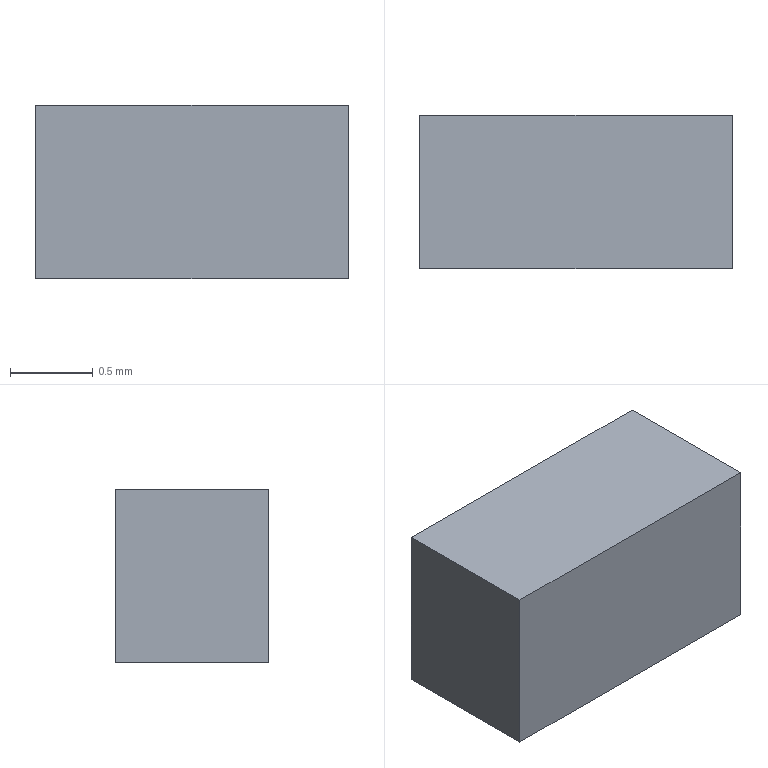Part | Creo | 1 solid | 6 faces | box 1.889 x 0.9288 x 1.053 mm | volume 1.848 mm3 | plane 6
STEP:
#1=CARTESIAN_POINT('',(0.,0.,0.));
#2=DIRECTION('',(0.,0.,1.));
#3=DIRECTION('',(1.,0.,0.));
#4=AXIS2_PLACEMENT_3D('',#1,#2,#3);
#5=CARTESIAN_POINT('',(-0.9404,-0.4484,0.));
#6=VERTEX_POINT('',#5);
#7=CARTESIAN_POINT('',(0.9491,-0.4484,0.));
#8=VERTEX_POINT('',#7);
#9=CARTESIAN_POINT('',(-0.9404,-0.4484,0.));
#10=DIRECTION('',(1.,0.,0.));
#11=VECTOR('',#10,1.889);
#12=LINE('',#9,#11);
#13=EDGE_CURVE('',#6,#8,#12,.T.);
#14=ORIENTED_EDGE('',*,*,#13,.T.);
#15=CARTESIAN_POINT('',(0.9491,0.4804,0.));
#16=VERTEX_POINT('',#15);
#17=CARTESIAN_POINT('',(0.9491,-0.4484,0.));
#18=DIRECTION('',(0.,1.,0.));
#19=VECTOR('',#18,0.9288);
#20=LINE('',#17,#19);
#21=EDGE_CURVE('',#8,#16,#20,.T.);
#22=ORIENTED_EDGE('',*,*,#21,.T.);
#23=CARTESIAN_POINT('',(-0.9404,0.4804,0.));
#24=VERTEX_POINT('',#23);
#25=CARTESIAN_POINT('',(0.9491,0.4804,0.));
#26=DIRECTION('',(-1.,0.,0.));
#27=VECTOR('',#26,1.889);
#28=LINE('',#25,#27);
#29=EDGE_CURVE('',#16,#24,#28,.T.);
#30=ORIENTED_EDGE('',*,*,#29,.T.);
#31=CARTESIAN_POINT('',(-0.9404,0.4804,0.));
#32=DIRECTION('',(0.,-1.,0.));
#33=VECTOR('',#32,0.9288);
#34=LINE('',#31,#33);
#35=EDGE_CURVE('',#24,#6,#34,.T.);
#36=ORIENTED_EDGE('',*,*,#35,.T.);
#37=EDGE_LOOP('',(#14,#22,#30,#36));
#38=FACE_OUTER_BOUND('',#37,.F.);
#39=CARTESIAN_POINT('',(0.,0.,0.));
#40=DIRECTION('',(0.,0.,1.));
#41=DIRECTION('',(1.,0.,0.));
#42=AXIS2_PLACEMENT_3D('',#39,#40,#41);
#43=PLANE('',#42);
#44=ADVANCED_FACE('',(#38),#43,.F.);
#45=ORIENTED_EDGE('',*,*,#13,.F.);
#46=CARTESIAN_POINT('',(-0.9404,-0.4484,1.053));
#47=VERTEX_POINT('',#46);
#48=CARTESIAN_POINT('',(-0.9404,-0.4484,0.));
#49=DIRECTION('',(0.,0.,1.));
#50=VECTOR('',#49,1.053);
#51=LINE('',#48,#50);
#52=EDGE_CURVE('',#6,#47,#51,.T.);
#53=ORIENTED_EDGE('',*,*,#52,.T.);
#54=CARTESIAN_POINT('',(0.9491,-0.4484,1.053));
#55=VERTEX_POINT('',#54);
#56=CARTESIAN_POINT('',(-0.9404,-0.4484,1.053));
#57=DIRECTION('',(1.,0.,0.));
#58=VECTOR('',#57,1.889);
#59=LINE('',#56,#58);
#60=EDGE_CURVE('',#47,#55,#59,.T.);
#61=ORIENTED_EDGE('',*,*,#60,.T.);
#62=CARTESIAN_POINT('',(0.9491,-0.4484,0.));
#63=DIRECTION('',(0.,0.,1.));
#64=VECTOR('',#63,1.053);
#65=LINE('',#62,#64);
#66=EDGE_CURVE('',#8,#55,#65,.T.);
#67=ORIENTED_EDGE('',*,*,#66,.F.);
#68=EDGE_LOOP('',(#45,#53,#61,#67));
#69=FACE_OUTER_BOUND('',#68,.F.);
#70=CARTESIAN_POINT('',(-0.9404,-0.4484,0.));
#71=DIRECTION('',(0.,-1.,0.));
#72=DIRECTION('',(1.,0.,0.));
#73=AXIS2_PLACEMENT_3D('',#70,#71,#72);
#74=PLANE('',#73);
#75=ADVANCED_FACE('',(#69),#74,.T.);
#76=ORIENTED_EDGE('',*,*,#35,.F.);
#77=CARTESIAN_POINT('',(-0.9404,0.4804,1.053));
#78=VERTEX_POINT('',#77);
#79=CARTESIAN_POINT('',(-0.9404,0.4804,0.));
#80=DIRECTION('',(0.,0.,1.));
#81=VECTOR('',#80,1.053);
#82=LINE('',#79,#81);
#83=EDGE_CURVE('',#24,#78,#82,.T.);
#84=ORIENTED_EDGE('',*,*,#83,.T.);
#85=CARTESIAN_POINT('',(-0.9404,0.4804,1.053));
#86=DIRECTION('',(0.,-1.,0.));
#87=VECTOR('',#86,0.9288);
#88=LINE('',#85,#87);
#89=EDGE_CURVE('',#78,#47,#88,.T.);
#90=ORIENTED_EDGE('',*,*,#89,.T.);
#91=ORIENTED_EDGE('',*,*,#52,.F.);
#92=EDGE_LOOP('',(#76,#84,#90,#91));
#93=FACE_OUTER_BOUND('',#92,.F.);
#94=CARTESIAN_POINT('',(-0.9404,0.4804,0.));
#95=DIRECTION('',(-1.,0.,0.));
#96=DIRECTION('',(0.,-1.,0.));
#97=AXIS2_PLACEMENT_3D('',#94,#95,#96);
#98=PLANE('',#97);
#99=ADVANCED_FACE('',(#93),#98,.T.);
#100=ORIENTED_EDGE('',*,*,#29,.F.);
#101=CARTESIAN_POINT('',(0.9491,0.4804,1.053));
#102=VERTEX_POINT('',#101);
#103=CARTESIAN_POINT('',(0.9491,0.4804,0.));
#104=DIRECTION('',(0.,0.,1.));
#105=VECTOR('',#104,1.053);
#106=LINE('',#103,#105);
#107=EDGE_CURVE('',#16,#102,#106,.T.);
#108=ORIENTED_EDGE('',*,*,#107,.T.);
#109=CARTESIAN_POINT('',(0.9491,0.4804,1.053));
#110=DIRECTION('',(-1.,0.,0.));
#111=VECTOR('',#110,1.889);
#112=LINE('',#109,#111);
#113=EDGE_CURVE('',#102,#78,#112,.T.);
#114=ORIENTED_EDGE('',*,*,#113,.T.);
#115=ORIENTED_EDGE('',*,*,#83,.F.);
#116=EDGE_LOOP('',(#100,#108,#114,#115));
#117=FACE_OUTER_BOUND('',#116,.F.);
#118=CARTESIAN_POINT('',(0.9491,0.4804,0.));
#119=DIRECTION('',(0.,1.,0.));
#120=DIRECTION('',(-1.,0.,0.));
#121=AXIS2_PLACEMENT_3D('',#118,#119,#120);
#122=PLANE('',#121);
#123=ADVANCED_FACE('',(#117),#122,.T.);
#124=ORIENTED_EDGE('',*,*,#21,.F.);
#125=ORIENTED_EDGE('',*,*,#66,.T.);
#126=CARTESIAN_POINT('',(0.9491,-0.4484,1.053));
#127=DIRECTION('',(0.,1.,0.));
#128=VECTOR('',#127,0.9288);
#129=LINE('',#126,#128);
#130=EDGE_CURVE('',#55,#102,#129,.T.);
#131=ORIENTED_EDGE('',*,*,#130,.T.);
#132=ORIENTED_EDGE('',*,*,#107,.F.);
#133=EDGE_LOOP('',(#124,#125,#131,#132));
#134=FACE_OUTER_BOUND('',#133,.F.);
#135=CARTESIAN_POINT('',(0.9491,-0.4484,0.));
#136=DIRECTION('',(1.,0.,0.));
#137=DIRECTION('',(0.,1.,0.));
#138=AXIS2_PLACEMENT_3D('',#135,#136,#137);
#139=PLANE('',#138);
#140=ADVANCED_FACE('',(#134),#139,.T.);
#141=ORIENTED_EDGE('',*,*,#60,.F.);
#142=ORIENTED_EDGE('',*,*,#89,.F.);
#143=ORIENTED_EDGE('',*,*,#113,.F.);
#144=ORIENTED_EDGE('',*,*,#130,.F.);
#145=EDGE_LOOP('',(#141,#142,#143,#144));
#146=FACE_OUTER_BOUND('',#145,.F.);
#147=CARTESIAN_POINT('',(0.,0.,1.053));
#148=DIRECTION('',(0.,0.,1.));
#149=DIRECTION('',(1.,0.,0.));
#150=AXIS2_PLACEMENT_3D('',#147,#148,#149);
#151=PLANE('',#150);
#152=ADVANCED_FACE('',(#146),#151,.T.);
#153=CLOSED_SHELL('',(#44,#75,#99,#123,#140,#152));
#154=MANIFOLD_SOLID_BREP('',#153);
#155=(LENGTH_UNIT()NAMED_UNIT(*)SI_UNIT(.MILLI.,.METRE.));
#156=UNCERTAINTY_MEASURE_WITH_UNIT(LENGTH_MEASURE(0.0002354),#155,'','');
#157=(NAMED_UNIT(*)PLANE_ANGLE_UNIT()SI_UNIT($,.RADIAN.));
#158=PLANE_ANGLE_MEASURE_WITH_UNIT(PLANE_ANGLE_MEASURE(0.01745),#157);
#159=(CONVERSION_BASED_UNIT('DEGREE',#158)NAMED_UNIT(*)PLANE_ANGLE_UNIT());
#160=(NAMED_UNIT(*)SI_UNIT($,.STERADIAN.)SOLID_ANGLE_UNIT());
#161=(GEOMETRIC_REPRESENTATION_CONTEXT(3)GLOBAL_UNCERTAINTY_ASSIGNED_CONTEXT((#156))GLOBAL_UNIT_ASSIGNED_CONTEXT((#155,#159,#160))REPRESENTATION_CONTEXT('',''));
#162=ADVANCED_BREP_SHAPE_REPRESENTATION('',(#4,#154),#161);